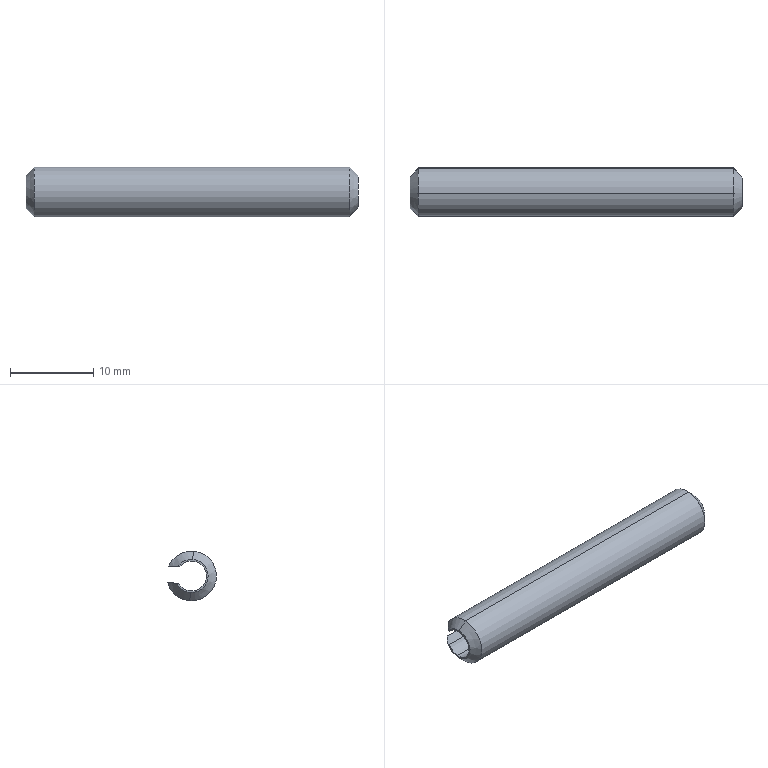Part | NX | features BREP 1 | 1 solid | 16 faces | box 40 x 5.893 x 6 mm | volume 608.896 mm3 | cylinder 6 | cone 6 | plane 4 | commonest cylinder face diameters 3.6 x3 6 x3
STEP:
#1=CARTESIAN_POINT('',(58.368,-53.471,-1.795));
#2=VERTEX_POINT('',#1);
#3=CARTESIAN_POINT('',(58.368,-53.729,1.795));
#4=VERTEX_POINT('',#3);
#5=CARTESIAN_POINT('',(58.368,-53.6,-0.000000274));
#6=DIRECTION('',(-1.,0.,0.));
#7=DIRECTION('',(0.,-0.07173,0.9974));
#8=AXIS2_PLACEMENT_3D('',#5,#6,#7);
#9=CIRCLE('',#8,1.8);
#10=EDGE_CURVE('',#2,#4,#9,.T.);
#11=ORIENTED_EDGE('',*,*,#10,.F.);
#12=CARTESIAN_POINT('',(18.368,-53.471,-1.795));
#13=VERTEX_POINT('',#12);
#14=CARTESIAN_POINT('',(58.368,-53.471,-1.795));
#15=DIRECTION('',(-1.,0.,0.));
#16=VECTOR('',#15,1000.);
#17=LINE('',#14,#16);
#18=EDGE_CURVE('',#2,#13,#17,.T.);
#19=ORIENTED_EDGE('',*,*,#18,.T.);
#20=CARTESIAN_POINT('',(18.368,-53.729,1.795));
#21=VERTEX_POINT('',#20);
#22=CARTESIAN_POINT('',(18.368,-53.6,-0.000000274));
#23=DIRECTION('',(-1.,0.,0.));
#24=DIRECTION('',(0.,-0.07173,0.9974));
#25=AXIS2_PLACEMENT_3D('',#22,#23,#24);
#26=CIRCLE('',#25,1.8);
#27=EDGE_CURVE('',#13,#21,#26,.T.);
#28=ORIENTED_EDGE('',*,*,#27,.T.);
#29=CARTESIAN_POINT('',(58.368,-53.729,1.795));
#30=DIRECTION('',(-1.,0.,0.));
#31=VECTOR('',#30,1000.);
#32=LINE('',#29,#31);
#33=EDGE_CURVE('',#4,#21,#32,.T.);
#34=ORIENTED_EDGE('',*,*,#33,.F.);
#35=EDGE_LOOP('',(#11,#19,#28,#34));
#36=FACE_BOUND('',#35,.T.);
#37=CARTESIAN_POINT('',(58.368,-53.6,-0.000000274));
#38=DIRECTION('',(-1.,0.,0.));
#39=DIRECTION('',(0.,0.07173,-0.9974));
#40=AXIS2_PLACEMENT_3D('',#37,#38,#39);
#41=CYLINDRICAL_SURFACE('',#40,1.8);
#42=ADVANCED_FACE('',(#36),#41,.F.);
#43=CARTESIAN_POINT('',(58.368,-52.179,1.105));
#44=VERTEX_POINT('',#43);
#45=CARTESIAN_POINT('',(58.368,-53.6,-0.000000274));
#46=DIRECTION('',(-1.,0.,0.));
#47=DIRECTION('',(0.,-0.07173,0.9974));
#48=AXIS2_PLACEMENT_3D('',#45,#46,#47);
#49=CIRCLE('',#48,1.8);
#50=EDGE_CURVE('',#4,#44,#49,.T.);
#51=ORIENTED_EDGE('',*,*,#50,.F.);
#52=ORIENTED_EDGE('',*,*,#33,.T.);
#53=CARTESIAN_POINT('',(18.368,-52.179,1.105));
#54=VERTEX_POINT('',#53);
#55=CARTESIAN_POINT('',(18.368,-53.6,-0.000000274));
#56=DIRECTION('',(-1.,0.,0.));
#57=DIRECTION('',(0.,-0.07173,0.9974));
#58=AXIS2_PLACEMENT_3D('',#55,#56,#57);
#59=CIRCLE('',#58,1.8);
#60=EDGE_CURVE('',#21,#54,#59,.T.);
#61=ORIENTED_EDGE('',*,*,#60,.T.);
#62=CARTESIAN_POINT('',(58.368,-52.179,1.105));
#63=DIRECTION('',(-1.,0.,0.));
#64=VECTOR('',#63,1000.);
#65=LINE('',#62,#64);
#66=EDGE_CURVE('',#44,#54,#65,.T.);
#67=ORIENTED_EDGE('',*,*,#66,.F.);
#68=EDGE_LOOP('',(#51,#52,#61,#67));
#69=FACE_BOUND('',#68,.T.);
#70=CARTESIAN_POINT('',(58.368,-53.6,-0.000000274));
#71=DIRECTION('',(-1.,0.,0.));
#72=DIRECTION('',(0.,0.07173,-0.9974));
#73=AXIS2_PLACEMENT_3D('',#70,#71,#72);
#74=CYLINDRICAL_SURFACE('',#73,1.8);
#75=ADVANCED_FACE('',(#69),#74,.F.);
#76=CARTESIAN_POINT('',(58.368,-53.457,-1.995));
#77=VERTEX_POINT('',#76);
#78=CARTESIAN_POINT('',(58.368,-51.801,-0.8732));
#79=VERTEX_POINT('',#78);
#80=CARTESIAN_POINT('',(58.368,-53.6,-0.000000274));
#81=DIRECTION('',(1.,0.,0.));
#82=DIRECTION('',(0.,0.07173,-0.9974));
#83=AXIS2_PLACEMENT_3D('',#80,#81,#82);
#84=CIRCLE('',#83,2.);
#85=EDGE_CURVE('',#77,#79,#84,.T.);
#86=ORIENTED_EDGE('',*,*,#85,.F.);
#87=CARTESIAN_POINT('',(57.368,-53.385,-2.992));
#88=VERTEX_POINT('',#87);
#89=CARTESIAN_POINT('',(57.368,-53.385,-2.992));
#90=DIRECTION('',(-0.7071,0.05072,-0.7053));
#91=VECTOR('',#90,1000.);
#92=LINE('',#89,#91);
#93=EDGE_CURVE('',#77,#88,#92,.T.);
#94=ORIENTED_EDGE('',*,*,#93,.T.);
#95=CARTESIAN_POINT('',(57.368,-50.707,-0.7945));
#96=VERTEX_POINT('',#95);
#97=CARTESIAN_POINT('',(57.368,-53.6,-0.000000274));
#98=DIRECTION('',(1.,0.,0.));
#99=DIRECTION('',(0.,0.07173,-0.9974));
#100=AXIS2_PLACEMENT_3D('',#97,#98,#99);
#101=CIRCLE('',#100,3.);
#102=EDGE_CURVE('',#88,#96,#101,.T.);
#103=ORIENTED_EDGE('',*,*,#102,.T.);
#104=CARTESIAN_POINT('',(57.368,-50.707,-0.7945));
#105=CARTESIAN_POINT('',(57.708,-51.066,-0.8204));
#106=CARTESIAN_POINT('',(58.044,-51.428,-0.8464));
#107=CARTESIAN_POINT('',(58.368,-51.801,-0.8732));
#108=B_SPLINE_CURVE_WITH_KNOTS('',3,(#104,#105,#106,#107),.UNSPECIFIED.,.F.,.F.,(4,4),(0.,0.001484),.UNSPECIFIED.);
#109=EDGE_CURVE('',#96,#79,#108,.T.);
#110=ORIENTED_EDGE('',*,*,#109,.T.);
#111=EDGE_LOOP('',(#86,#94,#103,#110));
#112=FACE_BOUND('',#111,.T.);
#113=CARTESIAN_POINT('',(57.368,-53.6,-0.000000274));
#114=DIRECTION('',(-1.,0.,0.));
#115=DIRECTION('',(0.,0.07173,-0.9974));
#116=AXIS2_PLACEMENT_3D('',#113,#114,#115);
#117=CONICAL_SURFACE('',#116,3.,0.7854);
#118=ADVANCED_FACE('',(#112),#117,.T.);
#119=ORIENTED_EDGE('',*,*,#93,.F.);
#120=CARTESIAN_POINT('',(58.368,-53.744,1.995));
#121=VERTEX_POINT('',#120);
#122=CARTESIAN_POINT('',(58.368,-53.6,-0.000000274));
#123=DIRECTION('',(1.,0.,0.));
#124=DIRECTION('',(0.,0.07173,-0.9974));
#125=AXIS2_PLACEMENT_3D('',#122,#123,#124);
#126=CIRCLE('',#125,2.);
#127=EDGE_CURVE('',#121,#77,#126,.T.);
#128=ORIENTED_EDGE('',*,*,#127,.F.);
#129=CARTESIAN_POINT('',(57.368,-53.816,2.992));
#130=VERTEX_POINT('',#129);
#131=CARTESIAN_POINT('',(57.368,-53.816,2.992));
#132=DIRECTION('',(-0.7071,-0.05072,0.7053));
#133=VECTOR('',#132,1000.);
#134=LINE('',#131,#133);
#135=EDGE_CURVE('',#121,#130,#134,.T.);
#136=ORIENTED_EDGE('',*,*,#135,.T.);
#137=CARTESIAN_POINT('',(57.368,-53.6,-0.000000274));
#138=DIRECTION('',(1.,0.,0.));
#139=DIRECTION('',(0.,0.07173,-0.9974));
#140=AXIS2_PLACEMENT_3D('',#137,#138,#139);
#141=CIRCLE('',#140,3.);
#142=EDGE_CURVE('',#130,#88,#141,.T.);
#143=ORIENTED_EDGE('',*,*,#142,.T.);
#144=EDGE_LOOP('',(#119,#128,#136,#143));
#145=FACE_BOUND('',#144,.T.);
#146=CARTESIAN_POINT('',(57.368,-53.6,-0.000000274));
#147=DIRECTION('',(-1.,0.,0.));
#148=DIRECTION('',(0.,0.07173,-0.9974));
#149=AXIS2_PLACEMENT_3D('',#146,#147,#148);
#150=CONICAL_SURFACE('',#149,3.,0.7854);
#151=ADVANCED_FACE('',(#145),#150,.T.);
#152=CARTESIAN_POINT('',(18.368,-51.944,1.122));
#153=VERTEX_POINT('',#152);
#154=CARTESIAN_POINT('',(18.368,-53.744,1.995));
#155=VERTEX_POINT('',#154);
#156=CARTESIAN_POINT('',(18.368,-53.6,-0.000000274));
#157=DIRECTION('',(1.,0.,0.));
#158=DIRECTION('',(0.,0.07173,-0.9974));
#159=AXIS2_PLACEMENT_3D('',#156,#157,#158);
#160=CIRCLE('',#159,2.);
#161=EDGE_CURVE('',#153,#155,#160,.T.);
#162=ORIENTED_EDGE('',*,*,#161,.T.);
#163=CARTESIAN_POINT('',(19.368,-53.816,2.992));
#164=VERTEX_POINT('',#163);
#165=CARTESIAN_POINT('',(18.368,-53.744,1.995));
#166=DIRECTION('',(0.7071,-0.05072,0.7053));
#167=VECTOR('',#166,1000.);
#168=LINE('',#165,#167);
#169=EDGE_CURVE('',#155,#164,#168,.T.);
#170=ORIENTED_EDGE('',*,*,#169,.T.);
#171=CARTESIAN_POINT('',(19.368,-50.851,1.2));
#172=VERTEX_POINT('',#171);
#173=CARTESIAN_POINT('',(19.368,-53.6,-0.000000274));
#174=DIRECTION('',(-1.,0.,0.));
#175=DIRECTION('',(0.,-0.07173,0.9974));
#176=AXIS2_PLACEMENT_3D('',#173,#174,#175);
#177=CIRCLE('',#176,3.);
#178=EDGE_CURVE('',#164,#172,#177,.T.);
#179=ORIENTED_EDGE('',*,*,#178,.T.);
#180=CARTESIAN_POINT('',(19.368,-50.851,1.2));
#181=CARTESIAN_POINT('',(19.029,-51.21,1.174));
#182=CARTESIAN_POINT('',(18.692,-51.571,1.148));
#183=CARTESIAN_POINT('',(18.368,-51.944,1.122));
#184=B_SPLINE_CURVE_WITH_KNOTS('',3,(#180,#181,#182,#183),.UNSPECIFIED.,.F.,.F.,(4,4),(0.,0.001484),.UNSPECIFIED.);
#185=EDGE_CURVE('',#172,#153,#184,.T.);
#186=ORIENTED_EDGE('',*,*,#185,.T.);
#187=EDGE_LOOP('',(#162,#170,#179,#186));
#188=FACE_BOUND('',#187,.T.);
#189=CARTESIAN_POINT('',(18.368,-53.6,-0.000000274));
#190=DIRECTION('',(1.,0.,0.));
#191=DIRECTION('',(0.,-0.07173,0.9974));
#192=AXIS2_PLACEMENT_3D('',#189,#190,#191);
#193=CONICAL_SURFACE('',#192,2.,0.7854);
#194=ADVANCED_FACE('',(#188),#193,.T.);
#195=ORIENTED_EDGE('',*,*,#169,.F.);
#196=CARTESIAN_POINT('',(18.368,-53.457,-1.995));
#197=VERTEX_POINT('',#196);
#198=CARTESIAN_POINT('',(18.368,-53.6,-0.000000274));
#199=DIRECTION('',(1.,0.,0.));
#200=DIRECTION('',(0.,0.07173,-0.9974));
#201=AXIS2_PLACEMENT_3D('',#198,#199,#200);
#202=CIRCLE('',#201,2.);
#203=EDGE_CURVE('',#155,#197,#202,.T.);
#204=ORIENTED_EDGE('',*,*,#203,.T.);
#205=CARTESIAN_POINT('',(19.368,-53.385,-2.992));
#206=VERTEX_POINT('',#205);
#207=CARTESIAN_POINT('',(18.368,-53.457,-1.995));
#208=DIRECTION('',(0.7071,0.05072,-0.7053));
#209=VECTOR('',#208,1000.);
#210=LINE('',#207,#209);
#211=EDGE_CURVE('',#197,#206,#210,.T.);
#212=ORIENTED_EDGE('',*,*,#211,.T.);
#213=CARTESIAN_POINT('',(19.368,-53.6,-0.000000274));
#214=DIRECTION('',(-1.,0.,0.));
#215=DIRECTION('',(0.,-0.07173,0.9974));
#216=AXIS2_PLACEMENT_3D('',#213,#214,#215);
#217=CIRCLE('',#216,3.);
#218=EDGE_CURVE('',#206,#164,#217,.T.);
#219=ORIENTED_EDGE('',*,*,#218,.T.);
#220=EDGE_LOOP('',(#195,#204,#212,#219));
#221=FACE_BOUND('',#220,.T.);
#222=CARTESIAN_POINT('',(18.368,-53.6,-0.000000274));
#223=DIRECTION('',(1.,0.,0.));
#224=DIRECTION('',(0.,-0.07173,0.9974));
#225=AXIS2_PLACEMENT_3D('',#222,#223,#224);
#226=CONICAL_SURFACE('',#225,2.,0.7854);
#227=ADVANCED_FACE('',(#221),#226,.T.);
#228=ORIENTED_EDGE('',*,*,#178,.F.);
#229=CARTESIAN_POINT('',(19.368,-53.816,2.992));
#230=DIRECTION('',(1.,0.,0.));
#231=VECTOR('',#230,1000.);
#232=LINE('',#229,#231);
#233=EDGE_CURVE('',#164,#130,#232,.T.);
#234=ORIENTED_EDGE('',*,*,#233,.T.);
#235=CARTESIAN_POINT('',(57.368,-50.851,1.2));
#236=VERTEX_POINT('',#235);
#237=CARTESIAN_POINT('',(57.368,-53.6,-0.000000274));
#238=DIRECTION('',(1.,0.,0.));
#239=DIRECTION('',(0.,0.07173,-0.9974));
#240=AXIS2_PLACEMENT_3D('',#237,#238,#239);
#241=CIRCLE('',#240,3.);
#242=EDGE_CURVE('',#236,#130,#241,.T.);
#243=ORIENTED_EDGE('',*,*,#242,.F.);
#244=CARTESIAN_POINT('',(19.368,-50.851,1.2));
#245=DIRECTION('',(-1.,0.,0.));
#246=VECTOR('',#245,1000.);
#247=LINE('',#244,#246);
#248=EDGE_CURVE('',#236,#172,#247,.T.);
#249=ORIENTED_EDGE('',*,*,#248,.T.);
#250=EDGE_LOOP('',(#228,#234,#243,#249));
#251=FACE_BOUND('',#250,.T.);
#252=CARTESIAN_POINT('',(19.368,-53.6,-0.000000274));
#253=DIRECTION('',(1.,0.,0.));
#254=DIRECTION('',(0.,-0.07173,0.9974));
#255=AXIS2_PLACEMENT_3D('',#252,#253,#254);
#256=CYLINDRICAL_SURFACE('',#255,3.);
#257=ADVANCED_FACE('',(#251),#256,.T.);
#258=ORIENTED_EDGE('',*,*,#233,.F.);
#259=ORIENTED_EDGE('',*,*,#218,.F.);
#260=CARTESIAN_POINT('',(19.368,-53.385,-2.992));
#261=DIRECTION('',(1.,0.,0.));
#262=VECTOR('',#261,1000.);
#263=LINE('',#260,#262);
#264=EDGE_CURVE('',#206,#88,#263,.T.);
#265=ORIENTED_EDGE('',*,*,#264,.T.);
#266=ORIENTED_EDGE('',*,*,#142,.F.);
#267=EDGE_LOOP('',(#258,#259,#265,#266));
#268=FACE_BOUND('',#267,.T.);
#269=CARTESIAN_POINT('',(19.368,-53.6,-0.000000274));
#270=DIRECTION('',(1.,0.,0.));
#271=DIRECTION('',(0.,-0.07173,0.9974));
#272=AXIS2_PLACEMENT_3D('',#269,#270,#271);
#273=CYLINDRICAL_SURFACE('',#272,3.);
#274=ADVANCED_FACE('',(#268),#273,.T.);
#275=ORIENTED_EDGE('',*,*,#264,.F.);
#276=CARTESIAN_POINT('',(19.368,-50.707,-0.7945));
#277=VERTEX_POINT('',#276);
#278=CARTESIAN_POINT('',(19.368,-53.6,-0.000000274));
#279=DIRECTION('',(-1.,0.,0.));
#280=DIRECTION('',(0.,-0.07173,0.9974));
#281=AXIS2_PLACEMENT_3D('',#278,#279,#280);
#282=CIRCLE('',#281,3.);
#283=EDGE_CURVE('',#277,#206,#282,.T.);
#284=ORIENTED_EDGE('',*,*,#283,.F.);
#285=CARTESIAN_POINT('',(19.368,-50.707,-0.7945));
#286=DIRECTION('',(1.,0.,0.));
#287=VECTOR('',#286,1000.);
#288=LINE('',#285,#287);
#289=EDGE_CURVE('',#277,#96,#288,.T.);
#290=ORIENTED_EDGE('',*,*,#289,.T.);
#291=ORIENTED_EDGE('',*,*,#102,.F.);
#292=EDGE_LOOP('',(#275,#284,#290,#291));
#293=FACE_BOUND('',#292,.T.);
#294=CARTESIAN_POINT('',(19.368,-53.6,-0.000000274));
#295=DIRECTION('',(1.,0.,0.));
#296=DIRECTION('',(0.,-0.07173,0.9974));
#297=AXIS2_PLACEMENT_3D('',#294,#295,#296);
#298=CYLINDRICAL_SURFACE('',#297,3.);
#299=ADVANCED_FACE('',(#293),#298,.T.);
#300=CARTESIAN_POINT('',(18.368,-52.036,-0.8901));
#301=VERTEX_POINT('',#300);
#302=CARTESIAN_POINT('',(18.368,-53.6,-0.000000274));
#303=DIRECTION('',(-1.,0.,0.));
#304=DIRECTION('',(0.,-0.07173,0.9974));
#305=AXIS2_PLACEMENT_3D('',#302,#303,#304);
#306=CIRCLE('',#305,1.8);
#307=EDGE_CURVE('',#301,#13,#306,.T.);
#308=ORIENTED_EDGE('',*,*,#307,.F.);
#309=CARTESIAN_POINT('',(18.368,-51.801,-0.8732));
#310=VERTEX_POINT('',#309);
#311=CARTESIAN_POINT('',(18.368,-52.036,-0.8901));
#312=DIRECTION('',(0.,-0.9974,-0.07173));
#313=VECTOR('',#312,1000.);
#314=LINE('',#311,#313);
#315=EDGE_CURVE('',#310,#301,#314,.T.);
#316=ORIENTED_EDGE('',*,*,#315,.F.);
#317=CARTESIAN_POINT('',(18.368,-53.6,-0.000000274));
#318=DIRECTION('',(1.,0.,0.));
#319=DIRECTION('',(0.,0.07173,-0.9974));
#320=AXIS2_PLACEMENT_3D('',#317,#318,#319);
#321=CIRCLE('',#320,2.);
#322=EDGE_CURVE('',#197,#310,#321,.T.);
#323=ORIENTED_EDGE('',*,*,#322,.F.);
#324=ORIENTED_EDGE('',*,*,#203,.F.);
#325=ORIENTED_EDGE('',*,*,#161,.F.);
#326=CARTESIAN_POINT('',(18.368,-52.179,1.105));
#327=DIRECTION('',(0.,0.9974,0.07173));
#328=VECTOR('',#327,1000.);
#329=LINE('',#326,#328);
#330=EDGE_CURVE('',#54,#153,#329,.T.);
#331=ORIENTED_EDGE('',*,*,#330,.F.);
#332=ORIENTED_EDGE('',*,*,#60,.F.);
#333=ORIENTED_EDGE('',*,*,#27,.F.);
#334=EDGE_LOOP('',(#308,#316,#323,#324,#325,#331,#332,#333));
#335=FACE_BOUND('',#334,.T.);
#336=CARTESIAN_POINT('',(18.368,-53.6,-0.000000274));
#337=DIRECTION('',(1.,0.,0.));
#338=DIRECTION('',(0.,-0.07173,0.9974));
#339=AXIS2_PLACEMENT_3D('',#336,#337,#338);
#340=PLANE('',#339);
#341=ADVANCED_FACE('',(#335),#340,.F.);
#342=ORIENTED_EDGE('',*,*,#211,.F.);
#343=ORIENTED_EDGE('',*,*,#322,.T.);
#344=CARTESIAN_POINT('',(18.368,-51.801,-0.8732));
#345=CARTESIAN_POINT('',(18.692,-51.428,-0.8464));
#346=CARTESIAN_POINT('',(19.029,-51.066,-0.8204));
#347=CARTESIAN_POINT('',(19.368,-50.707,-0.7945));
#348=B_SPLINE_CURVE_WITH_KNOTS('',3,(#344,#345,#346,#347),.UNSPECIFIED.,.F.,.F.,(4,4),(0.,0.001484),.UNSPECIFIED.);
#349=EDGE_CURVE('',#310,#277,#348,.T.);
#350=ORIENTED_EDGE('',*,*,#349,.T.);
#351=ORIENTED_EDGE('',*,*,#283,.T.);
#352=EDGE_LOOP('',(#342,#343,#350,#351));
#353=FACE_BOUND('',#352,.T.);
#354=CARTESIAN_POINT('',(18.368,-53.6,-0.000000274));
#355=DIRECTION('',(1.,0.,0.));
#356=DIRECTION('',(0.,-0.07173,0.9974));
#357=AXIS2_PLACEMENT_3D('',#354,#355,#356);
#358=CONICAL_SURFACE('',#357,2.,0.7854);
#359=ADVANCED_FACE('',(#353),#358,.T.);
#360=ORIENTED_EDGE('',*,*,#135,.F.);
#361=CARTESIAN_POINT('',(58.368,-51.944,1.122));
#362=VERTEX_POINT('',#361);
#363=CARTESIAN_POINT('',(58.368,-53.6,-0.000000274));
#364=DIRECTION('',(1.,0.,0.));
#365=DIRECTION('',(0.,0.07173,-0.9974));
#366=AXIS2_PLACEMENT_3D('',#363,#364,#365);
#367=CIRCLE('',#366,2.);
#368=EDGE_CURVE('',#362,#121,#367,.T.);
#369=ORIENTED_EDGE('',*,*,#368,.F.);
#370=CARTESIAN_POINT('',(58.368,-51.944,1.122));
#371=CARTESIAN_POINT('',(58.044,-51.571,1.148));
#372=CARTESIAN_POINT('',(57.708,-51.21,1.174));
#373=CARTESIAN_POINT('',(57.368,-50.851,1.2));
#374=B_SPLINE_CURVE_WITH_KNOTS('',3,(#370,#371,#372,#373),.UNSPECIFIED.,.F.,.F.,(4,4),(0.,0.001484),.UNSPECIFIED.);
#375=EDGE_CURVE('',#362,#236,#374,.T.);
#376=ORIENTED_EDGE('',*,*,#375,.T.);
#377=ORIENTED_EDGE('',*,*,#242,.T.);
#378=EDGE_LOOP('',(#360,#369,#376,#377));
#379=FACE_BOUND('',#378,.T.);
#380=CARTESIAN_POINT('',(57.368,-53.6,-0.000000274));
#381=DIRECTION('',(-1.,0.,0.));
#382=DIRECTION('',(0.,0.07173,-0.9974));
#383=AXIS2_PLACEMENT_3D('',#380,#381,#382);
#384=CONICAL_SURFACE('',#383,3.,0.7854);
#385=ADVANCED_FACE('',(#379),#384,.T.);
#386=ORIENTED_EDGE('',*,*,#368,.T.);
#387=ORIENTED_EDGE('',*,*,#127,.T.);
#388=ORIENTED_EDGE('',*,*,#85,.T.);
#389=CARTESIAN_POINT('',(58.368,-52.036,-0.8901));
#390=VERTEX_POINT('',#389);
#391=CARTESIAN_POINT('',(58.368,-53.529,-0.9974));
#392=DIRECTION('',(0.,-0.9974,-0.07173));
#393=VECTOR('',#392,1000.);
#394=LINE('',#391,#393);
#395=EDGE_CURVE('',#79,#390,#394,.T.);
#396=ORIENTED_EDGE('',*,*,#395,.T.);
#397=CARTESIAN_POINT('',(58.368,-53.6,-0.000000274));
#398=DIRECTION('',(-1.,0.,0.));
#399=DIRECTION('',(0.,-0.07173,0.9974));
#400=AXIS2_PLACEMENT_3D('',#397,#398,#399);
#401=CIRCLE('',#400,1.8);
#402=EDGE_CURVE('',#390,#2,#401,.T.);
#403=ORIENTED_EDGE('',*,*,#402,.T.);
#404=ORIENTED_EDGE('',*,*,#10,.T.);
#405=ORIENTED_EDGE('',*,*,#50,.T.);
#406=CARTESIAN_POINT('',(58.368,-52.179,1.105));
#407=DIRECTION('',(0.,0.9974,0.07173));
#408=VECTOR('',#407,1000.);
#409=LINE('',#406,#408);
#410=EDGE_CURVE('',#44,#362,#409,.T.);
#411=ORIENTED_EDGE('',*,*,#410,.T.);
#412=EDGE_LOOP('',(#386,#387,#388,#396,#403,#404,#405,#411));
#413=FACE_BOUND('',#412,.T.);
#414=CARTESIAN_POINT('',(58.368,-53.6,-0.000000274));
#415=DIRECTION('',(-1.,0.,0.));
#416=DIRECTION('',(0.,0.07173,-0.9974));
#417=AXIS2_PLACEMENT_3D('',#414,#415,#416);
#418=PLANE('',#417);
#419=ADVANCED_FACE('',(#413),#418,.F.);
#420=ORIENTED_EDGE('',*,*,#315,.T.);
#421=CARTESIAN_POINT('',(58.368,-52.036,-0.8901));
#422=DIRECTION('',(-1.,0.,0.));
#423=VECTOR('',#422,1000.);
#424=LINE('',#421,#423);
#425=EDGE_CURVE('',#390,#301,#424,.T.);
#426=ORIENTED_EDGE('',*,*,#425,.F.);
#427=ORIENTED_EDGE('',*,*,#395,.F.);
#428=ORIENTED_EDGE('',*,*,#109,.F.);
#429=ORIENTED_EDGE('',*,*,#289,.F.);
#430=ORIENTED_EDGE('',*,*,#349,.F.);
#431=EDGE_LOOP('',(#420,#426,#427,#428,#429,#430));
#432=FACE_BOUND('',#431,.T.);
#433=CARTESIAN_POINT('',(58.368,-52.036,-0.8901));
#434=DIRECTION('',(0.,0.07173,-0.9974));
#435=DIRECTION('',(1.,0.,0.));
#436=AXIS2_PLACEMENT_3D('',#433,#434,#435);
#437=PLANE('',#436);
#438=ADVANCED_FACE('',(#432),#437,.F.);
#439=ORIENTED_EDGE('',*,*,#248,.F.);
#440=ORIENTED_EDGE('',*,*,#375,.F.);
#441=ORIENTED_EDGE('',*,*,#410,.F.);
#442=ORIENTED_EDGE('',*,*,#66,.T.);
#443=ORIENTED_EDGE('',*,*,#330,.T.);
#444=ORIENTED_EDGE('',*,*,#185,.F.);
#445=EDGE_LOOP('',(#439,#440,#441,#442,#443,#444));
#446=FACE_BOUND('',#445,.T.);
#447=CARTESIAN_POINT('',(58.368,-52.179,1.105));
#448=DIRECTION('',(0.,-0.07173,0.9974));
#449=DIRECTION('',(-1.,0.,0.));
#450=AXIS2_PLACEMENT_3D('',#447,#448,#449);
#451=PLANE('',#450);
#452=ADVANCED_FACE('',(#446),#451,.F.);
#453=ORIENTED_EDGE('',*,*,#18,.F.);
#454=ORIENTED_EDGE('',*,*,#402,.F.);
#455=ORIENTED_EDGE('',*,*,#425,.T.);
#456=ORIENTED_EDGE('',*,*,#307,.T.);
#457=EDGE_LOOP('',(#453,#454,#455,#456));
#458=FACE_BOUND('',#457,.T.);
#459=CARTESIAN_POINT('',(58.368,-53.6,-0.000000274));
#460=DIRECTION('',(-1.,0.,0.));
#461=DIRECTION('',(0.,0.07173,-0.9974));
#462=AXIS2_PLACEMENT_3D('',#459,#460,#461);
#463=CYLINDRICAL_SURFACE('',#462,1.8);
#464=ADVANCED_FACE('',(#458),#463,.F.);
#465=CLOSED_SHELL('',(#42,#75,#118,#151,#194,#227,#257,#274,#299,#341,#359,#385,#419,#438,#452,#464));
#466=MANIFOLD_SOLID_BREP('',#465);
#467=(LENGTH_UNIT()NAMED_UNIT(*)SI_UNIT(.MILLI.,.METRE.));
#468=UNCERTAINTY_MEASURE_WITH_UNIT(LENGTH_MEASURE(0.0508),#467,'','');
#469=(NAMED_UNIT(*)PLANE_ANGLE_UNIT()SI_UNIT($,.RADIAN.));
#470=(NAMED_UNIT(*)SI_UNIT($,.STERADIAN.)SOLID_ANGLE_UNIT());
#471=(GEOMETRIC_REPRESENTATION_CONTEXT(3)GLOBAL_UNCERTAINTY_ASSIGNED_CONTEXT((#468))GLOBAL_UNIT_ASSIGNED_CONTEXT((#467,#469,#470))REPRESENTATION_CONTEXT('',''));
#472=ADVANCED_BREP_SHAPE_REPRESENTATION('',(#466),#471);